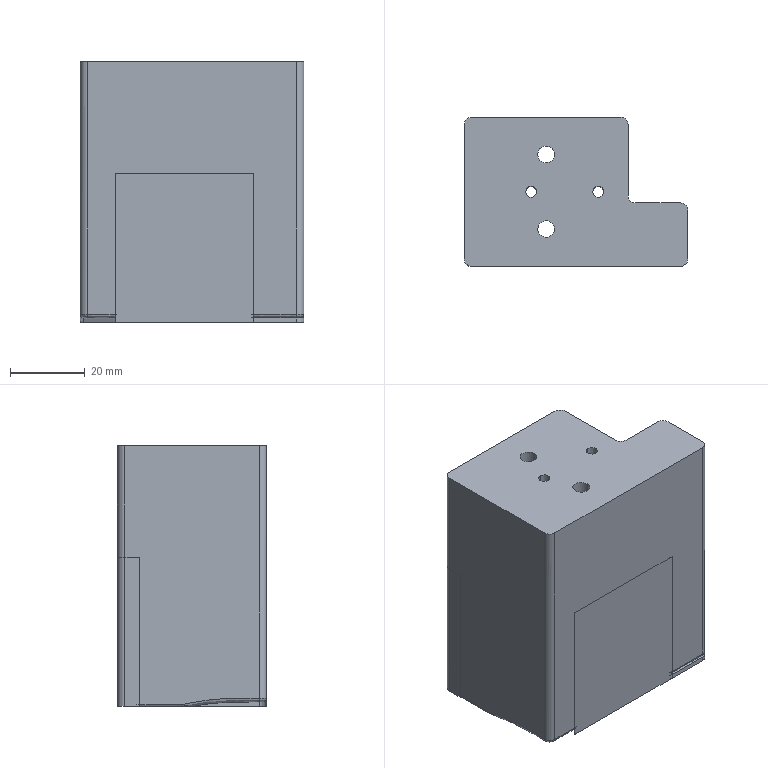NC program | NX | posted with a generic post | part box 60.004 x 40.015 x 70 mm
Lines 4655 to 5666 of 35085:
(FIXED_CONTOUR , TOOL : D6R0.5)
N9290 T08 M6
N9292 G54
N9294 G17 G0 G90 X-24.792 Y-19.73 B0. C0. S9500 M3
N9296 G43 Z30. H8
N9298 Z3.6
N9300 G94 G1 Z-1.5 F1000.
N9302 G3 X-25.319 Y-19.443 R0.6
N9304 G1 X-25.382 Y-19.444 Z-1.4 F2500.
N9306 X-25.523 Y-19.449
N9308 X-25.825 Y-19.453
N9310 X-26.015 Y-19.443
N9312 X-26.027 Z-1.5
N9314 X-26.04 Y-19.442
N9316 X-26.017 Z-1.304
N9318 X-26.005 Y-19.443 Z-1.3
N9320 X-25.825 Y-19.452
N9322 X-25.523 Y-19.449
N9324 X-25.386 Y-19.444
N9326 X-25.361 Y-19.443 Z-1.303
N9328 X-25.315 Y-19.442 Z-1.428
N9330 X-25.306 Z-1.5
N9332 X-25.292
N9334 X-25.31 Z-1.356
N9336 X-25.34 Z-1.205
N9338 X-25.391 Y-19.444 Z-1.2
N9340 X-25.523 Y-19.448
N9342 X-25.825 Y-19.452
N9344 X-26.005 Y-19.442
N9346 X-26.019 Z-1.211
N9348 X-26.053 Z-1.5
N9350 X-26.064
N9352 X-26.061 Z-1.465
N9354 X-26.021 Z-1.124
N9356 X-26.005 Z-1.1
N9358 X-25.825 Y-19.451
N9360 X-25.523 Y-19.448
N9362 X-25.364 Y-19.443 Z-1.102
N9364 X-25.325 Y-19.442 Z-1.131
N9366 X-25.283 Z-1.465
N9368 X-25.28 Z-1.5
N9370 X-25.272 Y-19.441
N9372 X-25.283 Z-1.356
N9374 X-25.316 Z-1.09
N9376 X-25.375 Y-19.443 Z-1.001
N9378 X-25.523 Y-19.447 Z-1.
N9380 X-25.825 Y-19.451
N9382 X-26.005 Y-19.442
N9384 X-26.025 Y-19.441 Z-1.043
N9386 X-26.061 Z-1.357
N9388 X-26.071 Z-1.5
N9390 X-26.166 Y-19.436
N9392 X-26.125 Z-1.045
N9394 X-26.114 Y-19.437 Z-0.999
N9396 X-26.079 Y-19.438 Z-0.933
N9398 X-26.061 Y-19.437 Z-0.918
N9400 X-26.015 Y-19.438 Z-0.901
N9402 X-25.764 Y-19.446 Z-0.9
N9404 X-25.523 Y-19.444
N9406 X-25.379 Y-19.439 Z-0.901
N9408 X-25.302 Y-19.44 Z-0.932
N9410 X-25.282 Z-0.96
N9412 X-25.194 Y-19.436 Z-1.297
N9414 X-25.179 Z-1.5
N9416 X-25.042 Y-19.428
N9418 X-24.995 Y-19.424
N9420 X-25. Z-1.403
N9422 X-25.07 Y-19.43 Z-1.401
N9424 X-25.09 Z-1.34
N9426 X-25.11 Y-19.431 Z-1.223
N9428 X-25.184 Y-19.434 Z-0.94
N9430 X-25.207 Y-19.43 Z-0.893
N9432 X-25.283 Y-19.427 Z-0.833
N9434 X-25.31 Y-19.426 Z-0.822
N9436 X-25.4 Y-19.427 Z-0.801
N9438 X-25.523 Y-19.431
N9440 X-25.825 Y-19.432
N9442 X-26.005 Y-19.426
N9444 X-26.049 Y-19.425 Z-0.808
N9446 X-26.106 Y-19.424 Z-0.829
N9448 X-26.125 Y-19.425 Z-0.842
N9450 X-26.163 Y-19.428 Z-0.881
N9452 X-26.189 Y-19.433 Z-0.927
N9454 X-26.209 Y-19.432 Z-0.966
N9456 X-26.224 Y-19.431 Z-1.032
N9458 X-26.246 Z-1.262
N9460 X-26.267 Y-19.43 Z-1.401
N9462 X-26.288 Y-19.428 Z-1.402
N9464 X-26.352 Y-19.424 Z-1.5
N9466 X-26.292 Y-19.428 Z-1.407
N9468 X-26.268 Z-0.932
N9470 X-26.246 Z-0.917
N9472 X-26.163 Z-0.88
N9474 X-26.125 Y-19.425 Z-0.842
N9476 X-26.104 Y-19.424 Z-0.828
N9478 X-26.049 Y-19.425 Z-0.808
N9480 X-26.005 Y-19.426 Z-0.801
N9482 X-25.946 Y-19.428
N9484 X-25.884 Z-0.783
N9486 X-25.812
N9488 X-25.516 Z-0.779
N9490 X-25.435 Z-0.801
N9492 X-25.4 Y-19.427
N9494 X-25.31 Y-19.426 Z-0.822
N9496 X-25.283 Y-19.427 Z-0.833
N9498 X-25.244 Y-19.428 Z-0.864
N9500 X-25.079 Z-0.947
N9502 X-25.046 Z-1.402
N9504 X-25. Y-19.424 Z-1.403
N9506 X-24.995 Z-1.5
N9508 X-24.957 Y-19.42
N9510 X-24.982 Z-0.949
N9512 X-25.042 Z-0.901
N9514 X-25.267 Z-0.791
N9516 X-25.403 Z-0.768
N9518 X-25.523 Z-0.752
N9520 X-25.884 Z-0.757
N9522 X-26.012 Z-0.77
N9524 X-26.075 Z-0.783
N9526 X-26.117 Z-0.803
N9528 X-26.125 Z-0.805
N9530 X-26.245 Z-0.856
N9532 X-26.31 Z-0.897
N9534 X-26.366 Z-0.937
N9536 X-26.379 Z-1.192
N9538 X-26.399 Z-1.5
N9540 X-26.495 Y-19.413
N9542 X-26.486 Z-1.315
N9544 X-26.463 Z-0.941
N9546 X-26.362 Z-0.87
N9548 X-26.245 Z-0.795
N9550 X-26.236 Z-0.791
N9552 X-26.005 Z-0.742
N9554 X-25.883 Z-0.73
N9556 X-25.74 Z-0.726
N9558 X-25.523
N9560 X-25.283 Z-0.76
N9562 X-25.119 Z-0.798
N9564 X-25.042 Z-0.836
N9566 X-24.9 Z-0.948
N9568 X-24.875 Z-1.5
N9570 X-24.782 Y-19.403
N9572 X-24.801 Z-0.946
N9574 X-24.981 Z-0.804
N9576 X-25.042 Z-0.782
N9578 X-25.293 Z-0.726
N9580 X-25.523 Z-0.697
N9582 X-25.872 Z-0.7
N9584 X-26.005 Z-0.711
N9586 X-26.245 Z-0.76
N9588 X-26.367 Z-0.799
N9590 X-26.426 Z-0.836
N9592 X-26.486 Z-0.879
N9594 X-26.555 Z-0.945
N9596 X-26.578 Z-1.5
N9598 X-26.676 Y-19.392
N9600 X-26.655 Z-0.95
N9602 X-26.507 Z-0.806
N9604 X-26.486 Z-0.797
N9606 X-26.256 Z-0.725
N9608 X-26.005 Z-0.679
N9610 X-25.852 Z-0.667
N9612 X-25.762 Z-0.665
N9614 X-25.523 Z-0.664
N9616 X-25.284 Z-0.694
N9618 X-25.042 Z-0.742
N9620 X-24.858 Z-0.808
N9622 X-24.802 Z-0.852
N9624 X-24.719 Z-0.945
N9626 X-24.701 Z-1.5
N9628 X-24.611 Y-19.38
N9630 X-24.629 Z-0.943
N9632 X-24.696 Z-0.868
N9634 X-24.763 Z-0.801
N9636 X-24.778 Z-0.795
N9638 X-24.804 Z-0.781
N9640 X-24.908 Z-0.743
N9642 X-25.042 Z-0.703
N9644 X-25.284 Z-0.656
N9646 X-25.523 Z-0.628
N9648 X-25.83 Z-0.629
N9650 X-25.882 Z-0.632
N9652 X-26.005 Z-0.643
N9654 X-26.244 Z-0.684
N9656 X-26.457 Z-0.741
N9658 X-26.486 Z-0.751
N9660 X-26.624 Z-0.811
N9662 X-26.727 Z-0.914
N9664 X-26.754 Z-0.953
N9666 X-26.769 Z-1.5
N9668 X-26.855 Y-19.366
N9670 X-26.841 Z-0.95
N9672 X-26.759 Z-0.834
N9674 X-26.742 Z-0.813
N9676 X-26.725 Z-0.802
N9678 X-26.606 Z-0.749
N9680 X-26.486 Z-0.705
N9682 X-26.383 Z-0.677
N9684 X-26.243 Z-0.642
N9686 X-26.067 Z-0.612
N9688 X-26.006 Z-0.604
N9690 X-25.881 Z-0.597
N9692 X-25.523 Z-0.594
N9694 X-25.275 Z-0.616
N9696 X-25.042 Z-0.659
N9698 X-24.806 Z-0.73
N9700 X-24.783 Z-0.74
N9702 X-24.732 Z-0.768
N9704 X-24.687 Z-0.785
N9706 X-24.529 Z-0.942
N9708 X-24.513 Z-1.5
N9710 X-24.414 Y-19.352
N9712 X-24.431 Z-0.944
N9714 X-24.483 Z-0.887
N9716 X-24.607 Z-0.768
N9718 X-24.682 Z-0.739
N9720 X-24.719 Z-0.719
N9722 X-24.808 Z-0.682
N9724 X-24.973 Z-0.633
N9726 X-25.042 Z-0.619
N9728 X-25.284 Z-0.586
N9730 X-25.523 Z-0.566
N9732 X-25.881 Z-0.569
N9734 X-26.016 Z-0.577
N9736 X-26.243 Z-0.605
N9738 X-26.378 Z-0.63
N9740 X-26.486 Z-0.658
N9742 X-26.723 Z-0.744
N9744 X-26.737 Z-0.751
N9746 X-26.785 Z-0.784
N9748 X-26.816 Z-0.798
N9750 X-26.912 Z-0.916
N9752 X-26.934 Z-0.948
N9754 X-26.948 Z-1.5
N9756 X-27.037 Y-19.337
N9758 X-27.031 Z-1.353
N9760 X-27.021 Z-0.944
N9762 X-26.89 Z-0.783
N9764 X-26.834 Z-0.758
N9766 X-26.798 Z-0.734
N9768 X-26.72 Z-0.695
N9770 X-26.583 Z-0.646
N9772 X-26.486 Z-0.621
N9774 X-26.242 Z-0.577
N9776 X-26.005 Z-0.548
N9778 X-25.851 Z-0.541
N9780 X-25.523 Z-0.539
N9782 X-25.285 Z-0.558
N9784 X-25.042 Z-0.59
N9786 X-24.81 Z-0.637
N9788 X-24.782 Z-0.645
N9790 X-24.655 Z-0.698
N9792 X-24.633 Z-0.71
N9794 X-24.56 Z-0.738
N9796 X-24.514 Z-0.762
N9798 X-24.424 Z-0.846
N9800 X-24.333 Z-0.946
N9802 X-24.316 Z-1.5
N9804 X-24.233 Y-19.321
N9806 X-24.246 Z-0.945
N9808 X-24.321 Z-0.84
N9810 X-24.358 Z-0.799
N9812 X-24.389 Z-0.77
N9814 X-24.56 Z-0.684
N9816 X-24.613 Z-0.663
N9818 X-24.812 Z-0.603
N9820 X-25.042 Z-0.557
N9822 X-25.285 Z-0.526
N9824 X-25.523 Z-0.508
N9826 X-25.88 Z-0.51
N9828 X-26.037 Z-0.52
N9830 X-26.241 Z-0.544
N9832 X-26.486 Z-0.588
N9834 X-26.718 Z-0.645
N9836 X-26.761 Z-0.662
N9838 X-26.868 Z-0.715
N9840 X-26.889 Z-0.729
N9842 X-26.975 Z-0.768
N9844 X-27.117 Z-0.94
N9846 X-27.122 Z-1.141
N9848 X-27.135 Z-1.5
N9850 X-27.231 Y-19.303
N9852 X-27.214 Z-0.935
N9854 X-27.086 Z-0.776
N9856 X-26.968 Z-0.709
N9858 X-26.911 Z-0.68
N9860 X-26.715 Z-0.608
N9862 X-26.606 Z-0.583
N9864 X-26.486 Z-0.553
N9866 X-26.218 Z-0.508
N9868 X-26.005 Z-0.484
N9870 X-25.879 Z-0.477
N9872 X-25.761 Z-0.475
N9874 X-25.523
N9876 X-25.285 Z-0.493
N9878 X-25.042 Z-0.523
N9880 X-24.815 Z-0.567
N9882 X-24.639 Z-0.62
N9884 X-24.56 Z-0.641
N9886 X-24.456 Z-0.68
N9888 X-24.323 Z-0.746
N9890 X-24.274 Z-0.779
N9892 X-24.24 Z-0.83
N9894 X-24.16 Z-0.943
N9896 X-24.147 Z-1.5
N9898 X-24.052 Y-19.283
N9900 X-24.062 Z-0.942
N9902 X-24.079 Z-0.909
N9904 X-24.157 Z-0.791
N9906 X-24.291 Z-0.701
N9908 X-24.326 Z-0.683
N9910 X-24.56 Z-0.596
N9912 X-24.818 Z-0.526
N9914 X-24.963 Z-0.498
N9916 X-25.057 Z-0.485
N9918 X-25.304 Z-0.459
N9920 X-25.523 Z-0.446
N9922 X-25.878 Z-0.448
N9924 X-26.012 Z-0.453
N9926 X-26.24 Z-0.475
N9928 X-26.393 Z-0.497
N9930 X-26.486 Z-0.513
N9932 X-26.712 Z-0.564
N9934 X-26.853 Z-0.616
N9936 X-26.968 Z-0.654
N9938 X-27.011 Z-0.671
N9940 X-27.068 Z-0.7
N9942 X-27.212 Z-0.784
N9944 X-27.275 Z-0.891
N9946 X-27.308 Z-0.933
N9948 X-27.317 Z-1.246
N9950 X-27.322 Z-1.5
N9952 X-27.418 Y-19.263
N9954 X-27.406 Z-0.932
N9956 X-27.34 Z-0.847
N9958 X-27.3 Z-0.78
N9960 X-27.208 Z-0.712
N9962 X-27.079 Z-0.645
N9964 X-26.968 Z-0.602
N9966 X-26.764 Z-0.535
N9968 X-26.708 Z-0.52
N9970 X-26.486 Z-0.479
N9972 X-26.415 Z-0.471
N9974 X-26.239 Z-0.445
N9976 X-26.005 Z-0.425
N9978 X-25.848 Z-0.419
N9980 X-25.523 Z-0.418
N9982 X-25.286 Z-0.432
N9984 X-25.134 Z-0.448
N9986 X-25.042 Z-0.455
N9988 X-24.821 Z-0.489
N9990 X-24.602 Z-0.537
N9992 X-24.56 Z-0.549
N9994 X-24.329 Z-0.628
N9996 X-24.147 Z-0.726
N9998 X-24.079 Z-0.772
N10000 X-24.049 Z-0.797
N10002 X-23.992 Z-0.91
N10004 X-23.972 Z-0.944
N10006 X-23.962 Z-1.5
N10008 X-23.869 Y-19.241
N10010 X-23.879 Z-0.947
N10012 X-23.917 Z-0.884
N10014 X-23.963 Z-0.792
N10016 X-24.038 Z-0.729
N10018 X-24.079 Z-0.7
N10020 X-24.332 Z-0.572
N10022 X-24.524 Z-0.521
N10024 X-24.56 Z-0.509
N10026 X-24.667 Z-0.489
N10028 X-24.824 Z-0.454
N10030 X-24.954 Z-0.438
N10032 X-25.042 Z-0.424
N10034 X-25.287 Z-0.402
N10036 X-25.523 Z-0.389
N10038 X-25.876 Z-0.39
N10040 X-26.04 Z-0.398
N10042 X-26.238 Z-0.415
N10044 X-26.327 Z-0.427
N10046 X-26.486 Z-0.445
N10048 X-26.599 Z-0.467
N10050 X-26.705 Z-0.483
N10052 X-26.982 Z-0.558
N10054 X-27.04 Z-0.577
N10056 X-27.148 Z-0.618
N10058 X-27.197 Z-0.643
N10060 X-27.254 Z-0.682
N10062 X-27.296 Z-0.703
N10064 X-27.391 Z-0.776
N10066 X-27.407 Z-0.802
N10068 X-27.449 Z-0.857
N10070 X-27.503 Z-0.936
N10072 X-27.514 Z-1.5
N10074 X-27.612 Y-19.219
N10076 X-27.601 Z-0.944
N10078 X-27.546 Z-0.861
N10080 X-27.485 Z-0.773
N10082 X-27.381 Z-0.69
N10084 X-27.301 Z-0.652
N10086 X-27.22 Z-0.596
N10088 X-27.03 Z-0.533
N10090 X-26.968 Z-0.518
N10092 X-26.701 Z-0.445
N10094 X-26.486 Z-0.411
N10096 X-26.237 Z-0.383
N10098 X-26.007 Z-0.367
N10100 X-25.875 Z-0.362
N10102 X-25.523 Z-0.36
N10104 X-25.287 Z-0.372
N10106 X-25.042 Z-0.392
N10108 X-24.827 Z-0.419
N10110 X-24.56 Z-0.47
N10112 X-24.481 Z-0.495
N10114 X-24.335 Z-0.534
N10116 X-24.079 Z-0.631
N10118 X-23.961 Z-0.715
N10120 X-23.875 Z-0.787
N10122 X-23.84 Z-0.856
N10124 X-23.784 Z-0.95
N10126 X-23.774 Z-1.5
N10128 X-23.678 Y-19.196
N10130 X-23.688 Z-0.952
N10132 X-23.762 Z-0.828
N10134 X-23.786 Z-0.781
N10136 X-23.883 Z-0.701
N10138 X-23.965 Z-0.642
N10140 X-24.003 Z-0.618
N10142 X-24.079 Z-0.587
N10144 X-24.163 Z-0.561
N10146 X-24.339 Z-0.495
N10148 X-24.437 Z-0.469
N10150 X-24.529 Z-0.44
N10152 X-24.821 Z-0.39
N10154 X-25.042 Z-0.365
N10156 X-25.329 Z-0.344
N10158 X-25.523 Z-0.335
N10160 X-25.875 Z-0.336
N10162 X-26.051 Z-0.344
N10164 X-26.236 Z-0.357
N10166 X-26.486 Z-0.383
N10168 X-26.705 Z-0.413
N10170 X-26.751 Z-0.422
N10172 X-26.968 Z-0.482
N10174 X-27.078 Z-0.507
N10176 X-27.2 Z-0.547
N10178 X-27.294 Z-0.583
N10180 X-27.349 Z-0.621
N10182 X-27.46 Z-0.674
N10184 X-27.58 Z-0.773
N10186 X-27.674 Z-0.913
N10188 X-27.696 Z-0.943
N10190 X-27.699 Z-0.953
N10192 X-27.708 Z-1.5
N10194 X-27.8 Y-19.173
N10196 X-27.798 Z-1.207
N10198 X-27.794 Z-0.962
N10200 X-27.779 Z-0.912
N10202 X-27.681 Z-0.778
N10204 X-27.562 Z-0.676
N10206 X-27.509 Z-0.641
N10208 X-27.397 Z-0.589
N10210 X-27.369 Z-0.57
N10212 X-27.204 Z-0.507
N10214 X-27.127 Z-0.481
N10216 X-26.968 Z-0.444
N10218 X-26.856 Z-0.413
N10220 X-26.694 Z-0.384
N10222 X-26.486 Z-0.355
N10224 X-26.194 Z-0.326
N10226 X-25.962 Z-0.313
N10228 X-25.753 Z-0.309
N10230 X-25.523
N10232 X-25.288 Z-0.319
N10234 X-25.042 Z-0.337
N10236 X-24.805 Z-0.364
N10238 X-24.441 Z-0.428
N10240 X-24.342 Z-0.456
N10242 X-24.251 Z-0.49
N10244 X-24.079 Z-0.542
N10246 X-23.924 Z-0.606
N10248 X-23.846 Z-0.656
N10250 X-23.803 Z-0.686
N10252 X-23.695 Z-0.776
N10254 X-23.683 Z-0.8
N10256 X-23.594 Z-0.947
N10258 X-23.59 Z-0.956
N10260 X-23.583 Z-1.5
N10262 X-23.497 Y-19.15
N10264 X-23.499 Z-0.972
N10266 X-23.548 Z-0.838
N10268 X-23.597 Z-0.779
N10270 X-23.602 Z-0.77
N10272 X-23.724 Z-0.67
N10274 X-23.842 Z-0.593
N10276 X-24.079 Z-0.497
N10278 X-24.315 Z-0.423
N10280 X-24.35 Z-0.414
N10282 X-24.566 Z-0.375
N10284 X-24.792 Z-0.337
N10286 X-25.042 Z-0.309
N10288 X-25.288 Z-0.292
N10290 X-25.523 Z-0.283
N10292 X-25.873 Z-0.284
N10294 X-26.005 Z-0.288
N10296 X-26.235 Z-0.302
N10298 X-26.486 Z-0.327
N10300 X-26.727 Z-0.36
N10302 X-26.968 Z-0.406
N10304 X-27.176 Z-0.455
N10306 X-27.208 Z-0.465
N10308 X-27.447 Z-0.557
N10310 X-27.559 Z-0.608
N10312 X-27.657 Z-0.672
N10314 X-27.779 Z-0.778
N10316 X-27.837 Z-0.839
N10318 X-27.864 Z-0.88
N10320 X-27.892 Z-0.971
N10322 X-27.895 Z-1.5
N10324 X-27.992 Y-19.126
N10326 X-27.982 Z-0.949
N10328 X-27.931 Z-0.87
N10330 X-27.904 Z-0.812
N10332 X-27.892 Z-0.794
N10334 X-27.868 Z-0.769
N10336 X-27.832 Z-0.74
N10338 X-27.749 Z-0.669
N10340 X-27.681 Z-0.624
N10342 X-27.626 Z-0.593
N10344 X-27.534 Z-0.551
N10346 X-27.298 Z-0.459
N10348 X-27.229 Z-0.438
N10350 X-27.057 Z-0.398
N10352 X-26.772 Z-0.342
N10354 X-26.576 Z-0.315
N10356 X-26.531 Z-0.311
N10358 X-26.486 Z-0.305
N10360 X-26.281 Z-0.284
N10362 X-26.005 Z-0.268
N10364 X-25.71 Z-0.263
N10366 X-25.523
N10368 X-25.332 Z-0.271
N10370 X-25.131 Z-0.284
N10372 X-25.042 Z-0.288
N10374 X-24.748 Z-0.32
N10376 X-24.56 Z-0.351
N10378 X-24.516 Z-0.36
N10380 X-24.471 Z-0.366
N10382 X-24.275 Z-0.403
N10384 X-24.23 Z-0.414
N10386 X-24.079 Z-0.461
N10388 X-24.034 Z-0.479
N10390 X-23.99 Z-0.492
N10392 X-23.793 Z-0.572
N10394 X-23.749 Z-0.593
N10396 X-23.673 Z-0.642
N10398 X-23.597 Z-0.705
N10400 X-23.547 Z-0.75
N10402 X-23.523 Z-0.77
N10404 X-23.48 Z-0.823
N10406 X-23.467 Z-0.85
N10408 X-23.425 Z-0.966
N10410 X-23.423 Z-1.5
N10412 X-23.349 Y-19.102
N10414 X-23.352 Z-0.957
N10416 X-23.384 Z-0.869
N10418 X-23.409 Z-0.812
N10420 X-23.445 Z-0.77
N10422 X-23.465 Z-0.75
N10424 X-23.493 Z-0.729
N10426 X-23.597 Z-0.636
N10428 X-23.626 Z-0.612
N10430 X-23.654 Z-0.594
N10432 X-23.746 Z-0.551
N10434 X-23.895 Z-0.49
N10436 X-23.987 Z-0.462
N10438 X-24.079 Z-0.425
N10440 X-24.136 Z-0.407
N10442 X-24.244 Z-0.382
N10444 X-24.377 Z-0.358
N10446 X-24.468 Z-0.345
N10448 X-24.56 Z-0.326
N10450 X-24.703 Z-0.302
N10452 X-24.795 Z-0.292
N10454 X-24.915 Z-0.281
N10456 X-25.042 Z-0.267
N10458 X-25.225 Z-0.26
N10460 X-25.378 Z-0.249
N10462 X-25.523 Z-0.243
N10464 X-25.739 Z-0.244
N10466 X-26.005 Z-0.248
N10468 X-26.331 Z-0.268
N10470 X-26.486 Z-0.283
N10472 X-26.578 Z-0.296
N10474 X-26.67 Z-0.304
N10476 X-26.819 Z-0.324
N10478 X-26.968 Z-0.353
N10480 X-27.06 Z-0.374
N10482 X-27.152 Z-0.391
N10484 X-27.282 Z-0.422
N10486 X-27.392 Z-0.454
N10488 X-27.449 Z-0.476
N10490 X-27.568 Z-0.526
N10492 X-27.623 Z-0.546
N10494 X-27.694 Z-0.579
N10496 X-27.809 Z-0.644
N10498 X-27.846 Z-0.668
N10500 X-27.931 Z-0.739
N10502 X-27.96 Z-0.763
N10504 X-28.079 Z-0.945
N10506 X-28.089 Z-1.5
N10508 X-28.186 Y-19.079
N10510 X-28.175 Z-0.94
N10512 X-28.063 Z-0.767
N10514 X-27.935 Z-0.662
N10516 X-27.763 Z-0.565
N10518 X-27.712 Z-0.542
N10520 X-27.629 Z-0.511
N10522 X-27.474 Z-0.447
N10524 X-27.335 Z-0.405
N10526 X-27.246 Z-0.384
N10528 X-27.107 Z-0.359
N10530 X-26.968 Z-0.326
N10532 X-26.85 Z-0.304
N10534 X-26.765 Z-0.293
N10536 X-26.625 Z-0.281
N10538 X-26.486 Z-0.261
N10540 X-26.38 Z-0.251
N10542 X-26.005 Z-0.228
N10544 X-25.523 Z-0.224
N10546 X-25.424 Z-0.228
N10548 X-25.32 Z-0.235
N10550 X-25.042 Z-0.247
N10552 X-24.936 Z-0.259
N10554 X-24.797 Z-0.27
N10556 X-24.658 Z-0.285
N10558 X-24.56 Z-0.301
N10560 X-24.421 Z-0.33
N10562 X-24.282 Z-0.349
N10564 X-24.191 Z-0.366
N10566 X-24.054 Z-0.4
N10568 X-23.94 Z-0.445
N10570 X-23.801 Z-0.488
N10572 X-23.699 Z-0.529
N10574 X-23.597 Z-0.577
N10576 X-23.568 Z-0.593
N10578 X-23.44 Z-0.708
N10580 X-23.397 Z-0.74
N10582 X-23.366 Z-0.769
N10584 X-23.339 Z-0.802
N10586 X-23.302 Z-0.888
N10588 X-23.279 Z-0.949
N10590 X-23.275 Z-1.278
N10592 Z-1.5
N10594 X-23.201 Y-19.055
N10596 X-23.206 Z-0.941
N10598 X-23.219 Z-0.907
N10600 X-23.269 Z-0.792
N10602 X-23.288 Z-0.769
N10604 X-23.329 Z-0.73
N10606 X-23.386 Z-0.688
N10608 X-23.493 Z-0.592
N10610 X-23.532 Z-0.572
N10612 X-23.597 Z-0.533
N10614 X-23.652 Z-0.508
N10616 X-23.706 Z-0.485
N10618 X-23.892 Z-0.429
N10620 X-23.991 Z-0.389
N10622 X-24.079 Z-0.364
N10624 X-24.139 Z-0.35
N10626 X-24.188 Z-0.341
N10628 X-24.374 Z-0.314
N10630 X-24.56 Z-0.277
N10632 X-24.612 Z-0.268
N10634 X-24.799 Z-0.247
N10636 X-24.985 Z-0.232
N10638 X-25.042 Z-0.226
N10640 X-25.523 Z-0.204
N10642 X-26.005 Z-0.208
N10644 X-26.429 Z-0.234
N10646 X-26.486 Z-0.24
N10648 X-26.673 Z-0.266
N10650 X-26.859 Z-0.282
N10652 X-26.913 Z-0.289
N10654 X-26.968 Z-0.299
N10656 X-27.154 Z-0.343
N10658 X-27.341 Z-0.377
N10660 X-27.395 Z-0.391
N10662 X-27.449 Z-0.407
N10664 X-27.575 Z-0.447
N10666 X-27.69 Z-0.496
N10668 X-27.801 Z-0.537
N10670 X-27.831 Z-0.551
N10672 X-28.045 Z-0.671
N10674 X-28.126 Z-0.737
N10676 X-28.165 Z-0.771
N10678 X-28.271 Z-0.936
N10680 X-28.284 Z-1.5
N10682 X-28.381 Y-19.031
N10684 X-28.367 Z-0.932
N10686 X-28.268 Z-0.775
N10688 X-28.212 Z-0.726
N10690 X-28.155 Z-0.68
N10692 X-28.088 Z-0.64
N10694 X-27.89 Z-0.532
N10696 X-27.751 Z-0.481
N10698 X-27.665 Z-0.444
N10700 X-27.435 Z-0.371
N10702 X-27.202 Z-0.328
N10704 X-26.954 Z-0.271
N10706 X-26.72 Z-0.251
N10708 X-26.479 Z-0.217
N10710 X-26.005 Z-0.188
N10712 X-25.509 Z-0.185
N10714 X-25.036 Z-0.206
N10716 X-24.801 Z-0.224
N10718 X-24.56 Z-0.252
N10720 X-24.327 Z-0.299
N10722 X-24.079 Z-0.335
N10724 X-23.928 Z-0.379
N10726 X-23.845 Z-0.412
N10728 X-23.604 Z-0.486
N10730 X-23.485 Z-0.556
N10732 X-23.418 Z-0.59
N10734 X-23.332 Z-0.667
N10736 X-23.261 Z-0.72
N10738 X-23.209 Z-0.769
N10740 X-23.199 Z-0.781
N10742 X-23.133 Z-0.933
N10744 X-23.127 Z-1.5
N10746 X-23.056 Y-19.007
N10748 X-23.064 Z-0.932
N10750 X-23.129 Z-0.771
N10752 X-23.193 Z-0.709
N10754 X-23.279 Z-0.646
N10756 X-23.343 Z-0.588
N10758 X-23.438 Z-0.54
N10760 X-23.544 Z-0.477
N10762 X-23.597 Z-0.457
N10764 X-23.798 Z-0.396
N10766 X-23.865 Z-0.369
N10768 X-23.999 Z-0.33
N10770 X-24.079 Z-0.313
N10772 X-24.28 Z-0.284
N10774 X-24.48 Z-0.244
N10776 X-24.56 Z-0.233
N10778 X-24.803 Z-0.207
N10780 X-25.042 Z-0.189
N10782 X-25.523 Z-0.169
N10784 X-26.005 Z-0.173
N10786 X-26.406 Z-0.198
N10788 X-26.486 Z-0.201
N10790 X-26.566 Z-0.208
N10792 X-26.767 Z-0.236
N10794 X-26.968 Z-0.253
N10796 X-27.048 Z-0.265
N10798 X-27.249 Z-0.313
N10800 X-27.449 Z-0.349
N10802 X-27.526 Z-0.368
N10804 X-27.658 Z-0.412
N10806 X-27.755 Z-0.441
N10808 X-27.812 Z-0.465
N10810 X-27.977 Z-0.527
N10812 X-28.165 Z-0.629
N10814 X-28.264 Z-0.689
N10816 X-28.37 Z-0.779
N10818 X-28.463 Z-0.93
N10820 X-28.478 Z-1.5
N10822 X-28.575 Y-18.983
N10824 X-28.56 Z-0.93
N10826 X-28.466 Z-0.778
N10828 X-28.374 Z-0.697
N10830 X-28.241 Z-0.618
N10832 X-28.062 Z-0.522
N10834 X-27.845 Z-0.439
N10836 X-27.719 Z-0.4
N10838 X-27.617 Z-0.366
N10840 X-27.449 Z-0.325
N10842 X-27.296 Z-0.297
N10844 X-27.142 Z-0.261
N10846 X-27.055 Z-0.249
N10848 X-26.968 Z-0.234
N10850 X-26.814 Z-0.221
N10852 X-26.661 Z-0.199
N10854 X-26.573 Z-0.195
N10856 X-26.486 Z-0.185
N10858 X-26.312 Z-0.178
N10860 X-26.005 Z-0.159
N10862 X-25.523 Z-0.156
N10864 X-25.216 Z-0.169
N10866 X-25.042 Z-0.174
N10868 X-24.888 Z-0.186
N10870 X-24.805 Z-0.191
N10872 X-24.651 Z-0.208
N10874 X-24.56 Z-0.215
N10876 X-24.473 Z-0.228
N10878 X-24.386 Z-0.238
N10880 X-24.232 Z-0.269
N10882 X-24.079 Z-0.291
N10884 X-23.905 Z-0.329
N10886 X-23.802 Z-0.359
N10888 X-23.751 Z-0.379
N10890 X-23.597 Z-0.426
N10892 X-23.52 Z-0.458
N10894 X-23.482 Z-0.47
N10896 X-23.391 Z-0.524
N10898 X-23.269 Z-0.586
N10900 X-23.225 Z-0.625
N10902 X-23.126 Z-0.699
N10904 X-23.059 Z-0.775
N10906 X-22.995 Z-0.935
N10908 X-22.987 Z-1.5
N10910 X-22.917 Y-18.959
N10912 X-22.927 Z-0.937
N10914 X-22.988 Z-0.783
N10916 X-23.053 Z-0.706
N10918 X-23.116 Z-0.646
N10920 X-23.172 Z-0.605
N10922 X-23.194 Z-0.585
N10924 X-23.344 Z-0.508
N10926 X-23.419 Z-0.464
N10928 X-23.478 Z-0.444
N10930 X-23.597 Z-0.395
N10932 X-23.704 Z-0.363
N10934 X-23.739 Z-0.349
N10936 X-23.811 Z-0.328
N10938 X-24.079 Z-0.269
N10940 X-24.185 Z-0.254
N10942 X-24.292 Z-0.233
N10944 X-24.426 Z-0.217
N10946 X-24.56 Z-0.197
N10948 X-24.7 Z-0.186
N10950 X-24.807 Z-0.174
N10952 X-24.935 Z-0.168
N10954 X-25.042 Z-0.159
N10956 X-25.31 Z-0.151
N10958 X-25.523 Z-0.142
N10960 X-26.005 Z-0.145
N10962 X-26.218 Z-0.158
N10964 X-26.486 Z-0.169
N10966 X-26.621 Z-0.184
N10968 X-26.755 Z-0.191
N10970 X-26.861 Z-0.206
N10972 X-26.968 Z-0.215
N10974 X-27.102 Z-0.238
N10976 X-27.236 Z-0.257
N10978 X-27.343 Z-0.282
N10980 X-27.449 Z-0.302
N10982 X-27.707 Z-0.364
N10984 X-27.78 Z-0.388
N10986 X-27.935 Z-0.436
N10988 X-28.148 Z-0.517
N10990 X-28.318 Z-0.607
N10992 X-28.468 Z-0.695
N10994 X-28.557 Z-0.774
N10996 X-28.602 Z-0.84
N10998 X-28.658 Z-0.931
N11000 X-28.672 Z-1.5
N11002 X-28.769 Y-18.936
N11004 X-28.755 Z-0.931
N11006 X-28.722 Z-0.878
N11008 X-28.648 Z-0.769
N11010 X-28.554 Z-0.688
N11012 X-28.383 Z-0.59
N11014 X-28.233 Z-0.512
N11016 X-28.03 Z-0.436
N11018 X-27.798 Z-0.362
N11020 X-27.449 Z-0.278
N11022 X-27.39 Z-0.267
N11024 X-27.33 Z-0.253
N11026 X-27.149 Z-0.227
N11028 X-26.968 Z-0.196
N11030 X-26.908 Z-0.191
N11032 X-26.849 Z-0.183
N11034 X-26.668 Z-0.173
N11036 X-26.486 Z-0.153
N11038 X-26.124 Z-0.138
N11040 X-26.005 Z-0.131
N11042 X-25.523 Z-0.128
N11044 X-25.042 Z-0.144
N11046 X-24.809 Z-0.158
N11048 X-24.749 Z-0.164
N11050 X-24.56 Z-0.179
N11052 X-24.379 Z-0.207
N11054 X-24.198 Z-0.227
N11056 X-24.138 Z-0.239
N11058 X-24.079 Z-0.248
N11060 X-23.716 Z-0.327
N11062 X-23.677 Z-0.339
N11064 X-23.657 Z-0.347
N11066 X-23.597 Z-0.365
N11068 X-23.437 Z-0.43
N11070 X-23.357 Z-0.457
N11072 X-23.297 Z-0.493
N11074 X-23.116 Z-0.586
N11076 X-22.979 Z-0.716
N11078 X-22.917 Z-0.791
N11080 X-22.86 Z-0.939
N11082 X-22.852 Z-1.5
N11084 X-22.792 Y-18.912
N11086 X-22.8 Z-0.939
N11088 X-22.852 Z-0.793
N11090 X-22.906 Z-0.725
N11092 X-23.04 Z-0.594
N11094 X-23.084 Z-0.563
N11096 X-23.116 Z-0.545
N11098 X-23.25 Z-0.477
N11100 X-23.295 Z-0.45
N11102 X-23.395 Z-0.417
N11104 X-23.614 Z-0.328
N11106 X-24.104 Z-0.222
N11108 X-24.332 Z-0.196
N11110 X-24.56 Z-0.161
N11112 X-24.811 Z-0.141
N11114 X-25.042 Z-0.129
N11116 X-25.523 Z-0.114
N11118 X-26.005 Z-0.117
N11120 X-26.486 Z-0.138
N11122 X-26.715 Z-0.163
N11124 X-26.955 Z-0.176
N11126 X-27.196 Z-0.216
N11128 X-27.437 Z-0.252
N11130 X-27.902 Z-0.365
N11132 X-28.126 Z-0.436
N11134 X-28.318 Z-0.506
N11136 X-28.512 Z-0.607
N11138 X-28.64 Z-0.68
N11140 X-28.74 Z-0.765
N11142 X-28.852 Z-0.932
N11144 X-28.866 Z-1.5
N11146 X-28.963 Y-18.888
N11148 X-28.949 Z-0.933
N11150 X-28.831 Z-0.761
N11152 X-28.726 Z-0.673
N11154 X-28.641 Z-0.624
N11156 X-28.549 Z-0.575
N11158 X-28.395 Z-0.498
N11160 X-28.222 Z-0.436
N11162 X-27.972 Z-0.357
N11164 X-27.517 Z-0.247
N11166 X-27.449 Z-0.235
N11168 X-27.243 Z-0.206
N11170 X-27.037 Z-0.17
N11172 X-26.968 Z-0.163
N11174 X-26.762 Z-0.152
N11176 X-26.555 Z-0.129
N11178 X-26.486 Z-0.125
N11180 X-26.005 Z-0.106
N11182 X-25.523 Z-0.103
N11184 X-25.042 Z-0.117
N11186 X-24.775 Z-0.13
N11188 X-24.491 Z-0.154
N11190 X-24.285 Z-0.185
N11192 X-24.079 Z-0.208
N11194 X-24.01 Z-0.22
N11196 X-23.597 Z-0.31
N11198 X-23.542 Z-0.326
N11200 X-23.353 Z-0.403
N11202 X-23.232 Z-0.444
N11204 X-23.203 Z-0.461
N11206 X-23.116 Z-0.505
N11208 X-23.051 Z-0.543
N11210 X-22.959 Z-0.605
N11212 X-22.895 Z-0.669
N11214 X-22.845 Z-0.725
N11216 X-22.794 Z-0.79
N11218 X-22.74 Z-0.94
N11220 X-22.733 Z-1.5
N11222 X-22.674 Y-18.864
N11224 X-22.68 Z-0.941
N11226 X-22.735 Z-0.787
N11228 X-22.788 Z-0.72
N11230 X-22.818 Z-0.69
N11232 X-22.887 Z-0.612
N11234 X-23.018 Z-0.523
N11236 X-23.116 Z-0.466
N11238 X-23.17 Z-0.437
N11240 X-23.311 Z-0.39
N11242 X-23.467 Z-0.326
N11244 X-23.597 Z-0.289
N11246 X-23.916 Z-0.219
N11248 X-24.079 Z-0.192
N11250 X-24.238 Z-0.174
N11252 X-24.397 Z-0.15
N11254 X-24.56 Z-0.134
N11256 X-24.815 Z-0.116
N11258 X-25.042 Z-0.105
N11260 X-25.523 Z-0.093
N11262 X-26.005 Z-0.095
N11264 X-26.324 Z-0.108
N11266 X-26.486 Z-0.113
N11268 X-26.649 Z-0.124
N11270 X-26.809 Z-0.141
N11272 X-26.968 Z-0.15
N11274 X-27.131 Z-0.168
N11276 X-27.29 Z-0.195
N11278 X-27.449 Z-0.217
N11280 X-27.609 Z-0.246
N11282 X-28.048 Z-0.351
N11284 X-28.317 Z-0.436
N11286 X-28.51 Z-0.506
N11288 X-28.626 Z-0.564
N11290 X-28.812 Z-0.665
N11292 X-28.927 Z-0.762
N11294 X-29.046 Z-0.935
N11296 X-29.06 Z-1.5
N11298 X-29.155 Y-18.84
N11300 X-29.143 Z-0.936
N11302 X-29.037 Z-0.775
N11304 X-28.991 Z-0.733
N11306 X-28.897 Z-0.657